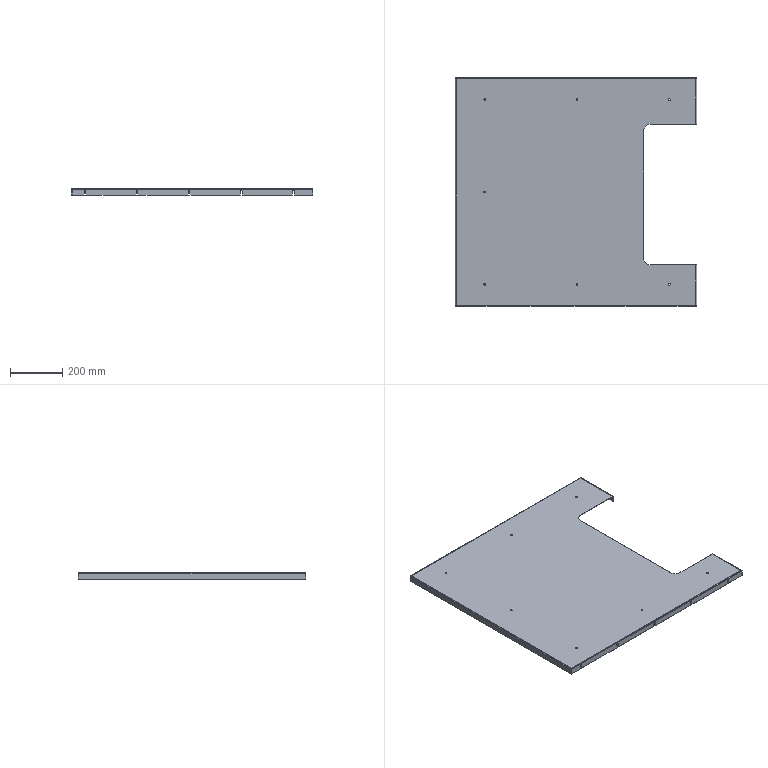Part | STEP file | SynoNew-0304-069 | 1 solid | 101 faces | box 928 x 876 x 25 mm | volume 1155671 mm3 | plane 70 | cylinder 31 | commonest cylinder face diameters 6.6 x17 3 x5 6 x5 10 x2 50 x2